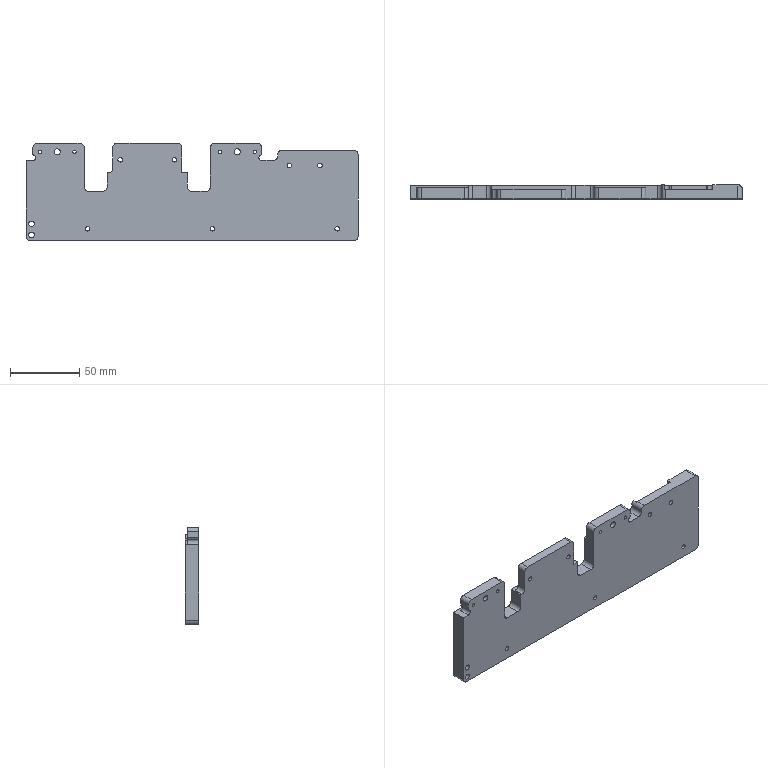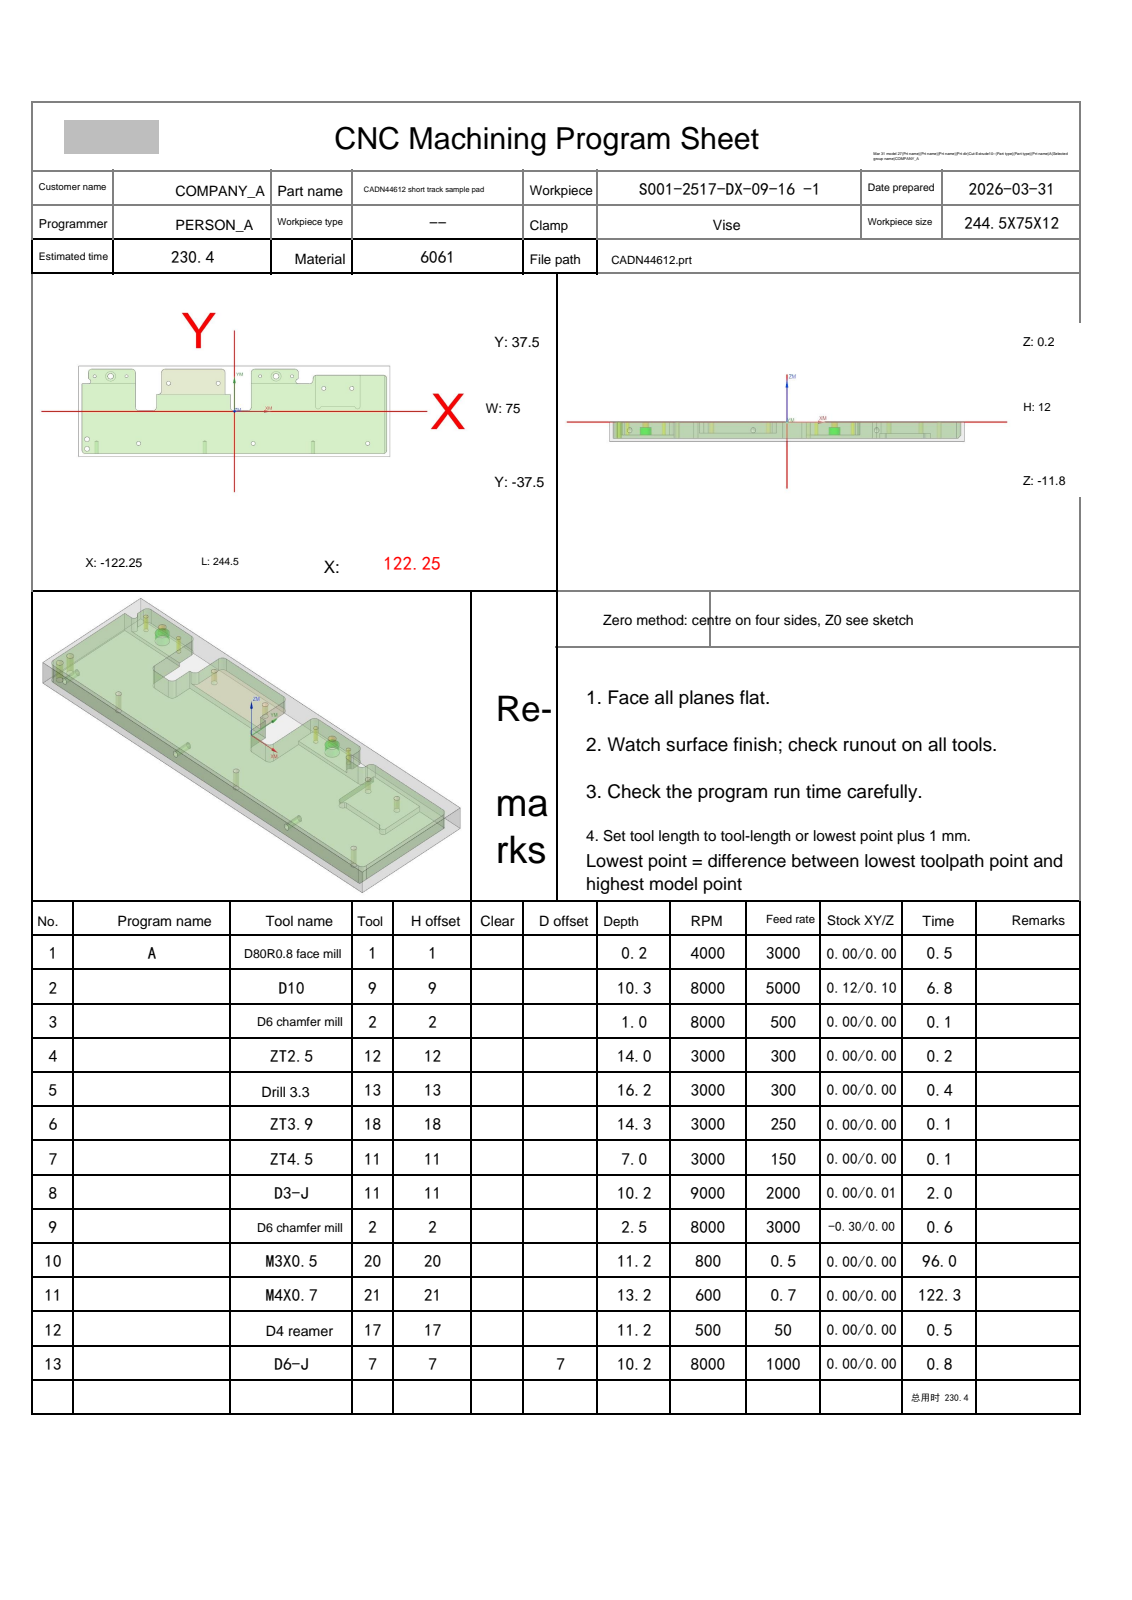NC program | NX | posted by the shop | part box 239.5 x 10 x 70 mm
Lines 1 to 2366 of 10745, first 1729 of 2364 lines:
%
O0001
(Machine time: 433.22 MIN)
(===Total Tool:11===)
(T1=D80R0.8 face mill D=80.  R=0.8  D-  H01 Z=0.    )
(T9=D10     D=10.  R=0.   D-  H09 Z=-10.1 )
(T2=D6 chamfer mill   D=6.   R=0.   D-  H02 Z=-2.3  )
(T12=ZT2.5  D=2.5  DR_a=118 D-  H12 Z=-13.75)
(T13=drill 3.3  D=3.3  DR_a=118 D-  H13 Z=-15.99)
(T18=ZT3.9  D=3.9  DR_a=120 D-  H18 Z=-14.13)
(T11=ZT4.5  D=4.5  DR_a=118 D-  H11 Z=-9.95 )
(T20=M3X0.5 D=2.5  DR_a=180 D-  H20 Z=-11.  )
(T21=M4X0.7 D=3.3  DR_a=180 D-  H21 Z=-13.  )
(T17=D4 reamer   D=4.   DR_a=180 D-  H17 Z=-11.  )
(T7=D6-J    D=6.   R=0.   D7  H07 Z=-10.  )
G80 G90 G17 G49 G40
G91 G28 Z0
M01
N1 T01 M06
(D80R0.8 face mill  D=80. R=0.8 H=01 ce=0.20 di=0.10)
G00 G90 G54 X164.75 Y0.0 M03 S4000
G43 H01 Z20.
M08
Z2.1
G01 Z.1 F3000.
X159.75
X-159.75
X-164.75
Z2.1
G00 Z20.
G00 G90 X164.75 Y0.0 M03 S4000
Z20.
Z2.
G01 Z0.0 F1000.
X159.75
X-159.75
X-164.75
Z2.
G00 Z20.
G91 G28 Z0.0
M05
M09
G91 G28 Z0.0
M01
N2 T09 M06
(D10  D=10. R=0. H=09 ce=0.12 di=0.10)
G00 G90 G54 X-74.5 Y49.5 M03 S8000
G43 H09 Z10.2
M08
Z.719
G01 Z-.481 F5000.
Y45.
G03 X-67.5 Y38. I7. J0.0
G01 X-61.641
G02 X-54.25 Y41.52 I7.391 J-6.
G01 X-10.25
G02 X-2.859 Y38. I0.0 J-9.52
G01 X5.734
G02 X6.734 Y37. I0.0 J-1.
G01 X6.72 Y36.833
X5.872 Y31.818
X5.858 Y31.651
G03 X6.294 Y30.826 I1. J0.0
G02 X6.73 Y30.004 I-.564 J-.826
G01 Y8.016
G02 X5.734 Y7.02 I-1. J.004
G01 X4.266
G02 X3.27 Y8.016 I.004 J1.
G01 Y14.
G03 X-.201 Y19.763 I-6.52 J0.0
G02 X-.73 Y20.641 I.471 J.882
G01 Y30.004
G02 X.266 Y31. I1. J-.004
G01 X2.45
G03 X3.421 Y31.762 I0.0 J1.
G01 X4.763 Y37.238
G02 X5.734 Y38. I.971 J-.238
G01 X8.859
G02 X16.25 Y41.52 I7.391 J-6.
G01 X47.25
G02 X54.641 Y38. I0.0 J-9.52
G01 X122.25
G02 X122.75 Y37.5 I0.0 J-.5
G01 Y34.391
G02 X126.27 Y27. I-6. J-7.391
G01 Y-32.065
G02 X116.75 Y-41.52 I-9.52 J.065
G01 X-116.75
G02 X-126.27 Y-32. I0.0 J9.52
G01 Y22.8
G02 X-122.75 Y28.589 I6.52 J0.0
G01 Y37.5
G02 X-122.25 Y38. I.5 J0.0
G01 X-119.141
G02 X-111.75 Y41.52 I7.391 J-6.
G01 X-80.75
G02 X-73.359 Y38. I0.0 J-9.52
G01 X-62.5
G02 X-61.5 Y37. I0.0 J-1.
X-61.537 Y36.729 I-1. J0.0
G01 X-63.733 Y28.927
G03 X-63.77 Y28.657 I.963 J-.271
G01 Y20.641
G02 X-64.299 Y19.763 I-1. J.004
G03 X-67.77 Y14. I3.049 J-5.763
G01 Y8.016
G02 X-68.766 Y7.02 I-1. J.004
G01 X-70.234
G02 X-71.23 Y8.016 I.004 J1.
G01 Y29.511
G03 X-71.675 Y30.215 I-.779 J0.0
G01 X-72.03 Y30.383
X-72.21 Y30.424
G03 X-72.63 Y30.004 I0.0 J-.42
G01 Y5.62
X-66.37
Y14.
G02 X-62.37 Y18.996 I5.12 J0.0
G01 Y32.
G02 X-54.25 Y40.12 I8.12 J0.0
G01 X-10.25
G02 X-2.13 Y32. I0.0 J-8.12
G01 Y18.996
G02 X1.87 Y14. I-1.12 J-4.996
G01 Y5.62
X8.13
Y32.
G02 X16.25 Y40.12 I8.12 J0.0
G01 X47.25
G02 X55.37 Y32. I0.0 J-8.12
G01 Y27.92
X56.682
G02 X64.75 Y35.12 I8.068 J-.92
G01 X116.75
G02 X124.87 Y27. I0.0 J-8.12
G01 Y-32.046
G02 X116.75 Y-40.12 I-8.12 J.046
G01 X-116.75
G02 X-124.87 Y-32. I0.0 J8.12
G01 Y22.8
G02 X-119.87 Y27.919 I5.12 J0.0
G01 Y32.
G02 X-111.75 Y40.12 I8.12 J0.0
G01 X-80.75
G02 X-72.63 Y32. I0.0 J-8.12
G01 Y30.004
G03 X-72.21 Y29.584 I.42 J0.0
G01 X-72.03 Y29.624
X-71.432 Y29.908
G03 X-71.211 Y30.192 I-.172 J.361
G02 X-70.234 Y31. I.981 J-.192
G01 X-64.766
G02 X-64.497 Y30.962 I-.004 J-1.
X-64.069 Y30.713 I-.273 J-.962
G01 Z.719
G00 Z3.
G01 X-74.5 Y49.5 F6000.
G00 Z.238
G01 Z-.962 F5000.
Y45.
G03 X-67.5 Y38. I7. J0.0
G01 X-61.641
G02 X-54.25 Y41.52 I7.391 J-6.
G01 X-10.25
G02 X-2.859 Y38. I0.0 J-9.52
G01 X5.734
G02 X6.734 Y37. I0.0 J-1.
G01 X6.72 Y36.833
X5.872 Y31.818
X5.858 Y31.651
G03 X6.294 Y30.826 I1. J0.0
G02 X6.73 Y30.004 I-.564 J-.826
G01 Y8.016
G02 X5.734 Y7.02 I-1. J.004
G01 X4.266
G02 X3.27 Y8.016 I.004 J1.
G01 Y14.
G03 X-.201 Y19.763 I-6.52 J0.0
G02 X-.73 Y20.641 I.471 J.882
G01 Y30.004
G02 X.266 Y31. I1. J-.004
G01 X2.45
G03 X3.421 Y31.762 I0.0 J1.
G01 X4.763 Y37.238
G02 X5.734 Y38. I.971 J-.238
G01 X8.859
G02 X16.25 Y41.52 I7.391 J-6.
G01 X47.25
G02 X54.641 Y38. I0.0 J-9.52
G01 X122.25
G02 X122.75 Y37.5 I0.0 J-.5
G01 Y34.391
G02 X126.27 Y27. I-6. J-7.391
G01 Y-32.065
G02 X116.75 Y-41.52 I-9.52 J.065
G01 X-116.75
G02 X-126.27 Y-32. I0.0 J9.52
G01 Y22.8
G02 X-122.75 Y28.589 I6.52 J0.0
G01 Y37.5
G02 X-122.25 Y38. I.5 J0.0
G01 X-119.141
G02 X-111.75 Y41.52 I7.391 J-6.
G01 X-80.75
G02 X-73.359 Y38. I0.0 J-9.52
G01 X-62.5
G02 X-61.5 Y37. I0.0 J-1.
X-61.537 Y36.729 I-1. J0.0
G01 X-63.733 Y28.927
G03 X-63.77 Y28.657 I.963 J-.27
G01 Y20.641
G02 X-64.299 Y19.763 I-1. J.004
G03 X-67.77 Y14. I3.049 J-5.763
G01 Y8.016
G02 X-68.766 Y7.02 I-1. J.004
G01 X-70.234
G02 X-71.23 Y8.016 I.004 J1.
G01 Y29.512
G03 X-71.675 Y30.215 I-.779 J0.0
G01 X-72.03 Y30.384
X-72.21 Y30.424
G03 X-72.63 Y30.004 I0.0 J-.42
G01 Y5.62
X-66.37
Y14.
G02 X-62.37 Y18.996 I5.12 J0.0
G01 Y32.
G02 X-54.25 Y40.12 I8.12 J0.0
G01 X-10.25
G02 X-2.13 Y32. I0.0 J-8.12
G01 Y18.996
G02 X1.87 Y14. I-1.12 J-4.996
G01 Y5.62
X8.13
Y32.
G02 X16.25 Y40.12 I8.12 J0.0
G01 X47.25
G02 X55.37 Y32. I0.0 J-8.12
G01 Y27.92
X56.682
G02 X64.75 Y35.12 I8.068 J-.92
G01 X116.75
G02 X124.87 Y27. I0.0 J-8.12
G01 Y-32.046
G02 X116.75 Y-40.12 I-8.12 J.046
G01 X-116.75
G02 X-124.87 Y-32. I0.0 J8.12
G01 Y22.8
G02 X-119.87 Y27.919 I5.12 J0.0
G01 Y32.
G02 X-111.75 Y40.12 I8.12 J0.0
G01 X-80.75
G02 X-72.63 Y32. I0.0 J-8.12
G01 Y30.004
G03 X-72.21 Y29.584 I.42 J0.0
G01 X-72.03 Y29.625
X-71.432 Y29.908
G03 X-71.211 Y30.192 I-.172 J.361
G02 X-70.234 Y31. I.981 J-.192
G01 X-64.766
G02 X-64.497 Y30.962 I-.004 J-1.
X-64.069 Y30.713 I-.273 J-.962
G01 Z.238
G00 Z2.519
G01 X-74.5 Y49.5 F6000.
G00 Z-.243
G01 Z-1.443 F5000.
Y45.
G03 X-67.5 Y38. I7. J0.0
G01 X-61.641
G02 X-54.25 Y41.52 I7.391 J-6.
G01 X-10.25
G02 X-2.859 Y38. I0.0 J-9.52
G01 X5.734
G02 X6.734 Y37. I0.0 J-1.
G01 X6.72 Y36.833
X5.873 Y31.817
X5.859 Y31.651
G03 X6.294 Y30.826 I1. J0.0
G02 X6.73 Y30.004 I-.564 J-.826
G01 Y8.016
G02 X5.734 Y7.02 I-1. J.004
G01 X4.266
G02 X3.27 Y8.016 I.004 J1.
G01 Y14.
G03 X-.202 Y19.764 I-6.52 J0.0
G02 X-.73 Y20.641 I.472 J.882
G01 Y30.004
G02 X.266 Y31. I1. J-.004
G01 X2.45
G03 X3.421 Y31.762 I0.0 J1.
G01 X4.763 Y37.238
G02 X5.734 Y38. I.971 J-.238
G01 X8.859
G02 X16.25 Y41.52 I7.391 J-6.
G01 X47.25
G02 X54.641 Y38. I0.0 J-9.52
G01 X122.25
G02 X122.75 Y37.5 I0.0 J-.5
G01 Y34.391
G02 X126.27 Y27. I-6. J-7.391
G01 Y-32.065
G02 X116.75 Y-41.52 I-9.52 J.065
G01 X-116.75
G02 X-126.27 Y-32. I0.0 J9.52
G01 Y22.8
G02 X-122.75 Y28.589 I6.52 J0.0
G01 Y37.5
G02 X-122.25 Y38. I.5 J0.0
G01 X-119.141
G02 X-111.75 Y41.52 I7.391 J-6.
G01 X-80.75
G02 X-73.359 Y38. I0.0 J-9.52
G01 X-62.5
G02 X-61.5 Y37. I0.0 J-1.
X-61.537 Y36.729 I-1. J0.0
G01 X-63.733 Y28.927
G03 X-63.77 Y28.657 I.963 J-.271
G01 Y20.641
G02 X-64.298 Y19.764 I-1. J.004
G03 X-67.77 Y14. I3.048 J-5.764
G01 Y8.016
G02 X-68.766 Y7.02 I-1. J.004
G01 X-70.234
G02 X-71.23 Y8.016 I.004 J1.
G01 Y29.512
G03 X-71.675 Y30.215 I-.779 J0.0
G01 X-72.03 Y30.384
X-72.21 Y30.424
G03 X-72.63 Y30.004 I0.0 J-.42
G01 Y5.62
X-66.37
Y14.
G02 X-62.37 Y18.996 I5.12 J0.0
G01 Y32.
G02 X-54.25 Y40.12 I8.12 J0.0
G01 X-10.25
G02 X-2.13 Y32. I0.0 J-8.12
G01 Y18.996
G02 X1.87 Y14. I-1.12 J-4.996
G01 Y5.62
X8.13
Y32.
G02 X16.25 Y40.12 I8.12 J0.0
G01 X47.25
G02 X55.37 Y32. I0.0 J-8.12
G01 Y27.92
X56.682
G02 X64.75 Y35.12 I8.068 J-.92
G01 X116.75
G02 X124.87 Y27. I0.0 J-8.12
G01 Y-32.046
G02 X116.75 Y-40.12 I-8.12 J.046
G01 X-116.75
G02 X-124.87 Y-32. I0.0 J8.12
G01 Y22.8
G02 X-119.87 Y27.919 I5.12 J0.0
G01 Y32.
G02 X-111.75 Y40.12 I8.12 J0.0
G01 X-80.75
G02 X-72.63 Y32. I0.0 J-8.12
G01 Y30.004
G03 X-72.21 Y29.584 I.42 J0.0
G01 X-72.03 Y29.625
X-71.432 Y29.909
G03 X-71.211 Y30.193 I-.172 J.361
G02 X-70.234 Y31. I.981 J-.193
G01 X-64.766
G02 X-64.497 Y30.962 I-.004 J-1.
X-64.069 Y30.713 I-.273 J-.962
G01 Z-.243
G00 Z2.038
G01 X-74.5 Y49.5 F6000.
G00 Z-.724
G01 Z-1.924 F5000.
Y45.
G03 X-67.5 Y38. I7. J0.0
G01 X-61.641
G02 X-54.25 Y41.52 I7.391 J-6.
G01 X-10.25
G02 X-2.859 Y38. I0.0 J-9.52
G01 X5.735
G02 X6.735 Y37. I0.0 J-1.
G01 X6.721 Y36.833
X5.873 Y31.817
X5.859 Y31.651
G03 X6.294 Y30.826 I1. J0.0
G02 X6.73 Y30.005 I-.564 J-.826
G01 Y8.015
G02 X5.735 Y7.02 I-1. J.005
G01 X4.265
G02 X3.27 Y8.015 I.005 J1.
G01 Y14.
G03 X-.202 Y19.764 I-6.52 J0.0
G02 X-.73 Y20.641 I.472 J.882
G01 Y30.005
G02 X.265 Y31. I1. J-.005
G01 X2.45
G03 X3.421 Y31.762 I0.0 J1.
G01 X4.763 Y37.238
G02 X5.735 Y38. I.971 J-.238
G01 X8.859
G02 X16.25 Y41.52 I7.391 J-6.
G01 X47.25
G02 X54.641 Y38. I0.0 J-9.52
G01 X122.25
G02 X122.75 Y37.5 I0.0 J-.5
G01 Y34.391
G02 X126.27 Y27. I-6. J-7.391
G01 Y-32.065
G02 X116.75 Y-41.52 I-9.52 J.065
G01 X-116.75
G02 X-126.27 Y-32. I0.0 J9.52
G01 Y22.8
G02 X-122.75 Y28.589 I6.52 J0.0
G01 Y37.5
G02 X-122.25 Y38. I.5 J0.0
G01 X-119.141
G02 X-111.75 Y41.52 I7.391 J-6.
G01 X-80.75
G02 X-73.359 Y38. I0.0 J-9.52
G01 X-62.5
G02 X-61.5 Y37. I0.0 J-1.
X-61.537 Y36.729 I-1. J0.0
G01 X-63.733 Y28.927
G03 X-63.77 Y28.657 I.963 J-.27
G01 Y20.641
G02 X-64.298 Y19.764 I-1. J.005
G03 X-67.77 Y14. I3.048 J-5.764
G01 Y8.015
G02 X-68.765 Y7.02 I-1. J.005
G01 X-70.235
G02 X-71.23 Y8.015 I.005 J1.
G01 Y29.512
G03 X-71.675 Y30.216 I-.779 J0.0
G01 X-72.03 Y30.384
X-72.21 Y30.425
G03 X-72.63 Y30.005 I0.0 J-.42
G01 Y5.62
X-66.37
Y14.
G02 X-62.37 Y18.996 I5.12 J0.0
G01 Y32.
G02 X-54.25 Y40.12 I8.12 J0.0
G01 X-10.25
G02 X-2.13 Y32. I0.0 J-8.12
G01 Y18.996
G02 X1.87 Y14. I-1.12 J-4.996
G01 Y5.62
X8.13
Y32.
G02 X16.25 Y40.12 I8.12 J0.0
G01 X47.25
G02 X55.37 Y32. I0.0 J-8.12
G01 Y27.92
X56.682
G02 X64.75 Y35.12 I8.068 J-.92
G01 X116.75
G02 X124.87 Y27. I0.0 J-8.12
G01 Y-32.046
G02 X116.75 Y-40.12 I-8.12 J.046
G01 X-116.75
G02 X-124.87 Y-32. I0.0 J8.12
G01 Y22.8
G02 X-119.87 Y27.919 I5.12 J0.0
G01 Y32.
G02 X-111.75 Y40.12 I8.12 J0.0
G01 X-80.75
G02 X-72.63 Y32. I0.0 J-8.12
G01 Y30.005
G03 X-72.21 Y29.585 I.42 J0.0
G01 X-72.03 Y29.625
X-71.432 Y29.909
G03 X-71.211 Y30.193 I-.172 J.361
G02 X-70.235 Y31. I.981 J-.193
G01 X-64.765
G02 X-64.497 Y30.962 I-.005 J-1.
X-64.069 Y30.713 I-.273 J-.962
G01 Z-.724
G00 Z1.557
G01 X-74.5 Y49.5 F6000.
G00 Z-1.205
G01 Z-2.405 F5000.
Y45.
G03 X-67.5 Y38. I7. J0.0
G01 X-61.641
G02 X-54.25 Y41.52 I7.391 J-6.
G01 X-10.25
G02 X-2.859 Y38. I0.0 J-9.52
G01 X5.735
G02 X6.735 Y37. I0.0 J-1.
G01 X6.721 Y36.833
X5.873 Y31.817
X5.859 Y31.651
G03 X6.294 Y30.826 I1. J0.0
G02 X6.73 Y30.005 I-.564 J-.826
G01 Y8.015
G02 X5.735 Y7.02 I-1. J.005
G01 X4.265
G02 X3.27 Y8.015 I.005 J1.
G01 Y14.
G03 X-.202 Y19.764 I-6.52 J0.0
G02 X-.73 Y20.64 I.472 J.882
G01 Y30.005
G02 X.265 Y31. I1. J-.005
G01 X2.451
G03 X3.422 Y31.762 I0.0 J1.
G01 X4.764 Y37.238
G02 X5.735 Y38. I.971 J-.238
G01 X8.859
G02 X16.25 Y41.52 I7.391 J-6.
G01 X47.25
G02 X54.641 Y38. I0.0 J-9.52
G01 X122.25
G02 X122.75 Y37.5 I0.0 J-.5
G01 Y34.391
G02 X126.27 Y27. I-6. J-7.391
G01 Y-32.065
G02 X116.75 Y-41.52 I-9.52 J.065
G01 X-116.75
G02 X-126.27 Y-32. I0.0 J9.52
G01 Y22.8
G02 X-122.75 Y28.589 I6.52 J0.0
G01 Y37.5
G02 X-122.25 Y38. I.5 J0.0
G01 X-119.141
G02 X-111.75 Y41.52 I7.391 J-6.
G01 X-80.75
G02 X-73.359 Y38. I0.0 J-9.52
G01 X-62.5
G02 X-61.5 Y37. I0.0 J-1.
X-61.537 Y36.729 I-1. J0.0
G01 X-63.733 Y28.927
G03 X-63.77 Y28.657 I.963 J-.27
G01 Y20.64
G02 X-64.298 Y19.764 I-1. J.005
G03 X-67.77 Y14. I3.048 J-5.764
G01 Y8.015
G02 X-68.765 Y7.02 I-1. J.005
G01 X-70.235
G02 X-71.23 Y8.015 I.005 J1.
G01 Y29.513
G03 X-71.675 Y30.216 I-.779 J0.0
G01 X-72.03 Y30.384
X-72.21 Y30.425
G03 X-72.63 Y30.005 I0.0 J-.42
G01 Y5.62
X-66.37
Y14.
G02 X-62.37 Y18.996 I5.12 J0.0
G01 Y32.
G02 X-54.25 Y40.12 I8.12 J0.0
G01 X-10.25
G02 X-2.13 Y32. I0.0 J-8.12
G01 Y18.996
G02 X1.87 Y14. I-1.12 J-4.996
G01 Y5.62
X8.13
Y32.
G02 X16.25 Y40.12 I8.12 J0.0
G01 X47.25
G02 X55.37 Y32. I0.0 J-8.12
G01 Y27.92
X56.682
G02 X64.75 Y35.12 I8.068 J-.92
G01 X116.75
G02 X124.87 Y27. I0.0 J-8.12
G01 Y-32.046
G02 X116.75 Y-40.12 I-8.12 J.046
G01 X-116.75
G02 X-124.87 Y-32. I0.0 J8.12
G01 Y22.8
G02 X-119.87 Y27.919 I5.12 J0.0
G01 Y32.
G02 X-111.75 Y40.12 I8.12 J0.0
G01 X-80.75
G02 X-72.63 Y32. I0.0 J-8.12
G01 Y30.005
G03 X-72.21 Y29.585 I.42 J0.0
G01 X-72.03 Y29.625
X-71.432 Y29.909
G03 X-71.211 Y30.193 I-.172 J.361
G02 X-70.235 Y31. I.981 J-.193
G01 X-64.765
G02 X-64.497 Y30.962 I-.005 J-1.
X-64.069 Y30.713 I-.273 J-.962
G01 Z-1.205
G00 Z1.076
G01 X-74.5 Y49.5 F6000.
G00 Z-1.686
G01 Z-2.886 F5000.
Y45.
G03 X-67.5 Y38. I7. J0.0
G01 X-61.641
G02 X-54.25 Y41.52 I7.391 J-6.
G01 X-10.25
G02 X-2.859 Y38. I0.0 J-9.52
G01 X5.735
G02 X6.735 Y37. I0.0 J-1.
G01 X6.721 Y36.833
X5.873 Y31.817
X5.859 Y31.651
G03 X6.294 Y30.826 I1. J0.0
G02 X6.73 Y30.005 I-.564 J-.825
G01 Y8.015
G02 X5.735 Y7.02 I-1. J.005
G01 X4.265
G02 X3.27 Y8.015 I.005 J1.
G01 Y14.
G03 X-.202 Y19.764 I-6.52 J0.0
G02 X-.73 Y20.64 I.472 J.881
G01 Y30.005
G02 X.265 Y31. I1. J-.005
G01 X2.451
G03 X3.422 Y31.762 I0.0 J1.
G01 X4.764 Y37.238
G02 X5.735 Y38. I.971 J-.238
G01 X8.859
G02 X16.25 Y41.52 I7.391 J-6.
G01 X47.25
G02 X54.641 Y38. I0.0 J-9.52
G01 X122.25
G02 X122.75 Y37.5 I0.0 J-.5
G01 Y34.391
G02 X126.27 Y27. I-6. J-7.391
G01 Y-32.065
G02 X116.75 Y-41.52 I-9.52 J.065
G01 X-116.75
G02 X-126.27 Y-32. I0.0 J9.52
G01 Y22.8
G02 X-122.75 Y28.589 I6.52 J0.0
G01 Y37.5
G02 X-122.25 Y38. I.5 J0.0
G01 X-119.141
G02 X-111.75 Y41.52 I7.391 J-6.
G01 X-80.75
G02 X-73.359 Y38. I0.0 J-9.52
G01 X-62.5
G02 X-61.5 Y37. I0.0 J-1.
X-61.537 Y36.729 I-1. J0.0
G01 X-63.733 Y28.927
G03 X-63.77 Y28.657 I.963 J-.271
G01 Y20.64
G02 X-64.298 Y19.764 I-1. J.005
G03 X-67.77 Y14. I3.048 J-5.764
G01 Y8.015
G02 X-68.765 Y7.02 I-1. J.005
G01 X-70.235
G02 X-71.23 Y8.015 I.005 J1.
G01 Y29.513
G03 X-71.675 Y30.216 I-.779 J0.0
G01 X-72.03 Y30.385
X-72.21 Y30.425
G03 X-72.63 Y30.005 I0.0 J-.42
G01 Y5.62
X-66.37
Y14.
G02 X-62.37 Y18.996 I5.12 J0.0
G01 Y32.
G02 X-54.25 Y40.12 I8.12 J0.0
G01 X-10.25
G02 X-2.13 Y32. I0.0 J-8.12
G01 Y18.996
G02 X1.87 Y14. I-1.12 J-4.996
G01 Y5.62
X8.13
Y32.
G02 X16.25 Y40.12 I8.12 J0.0
G01 X47.25
G02 X55.37 Y32. I0.0 J-8.12
G01 Y27.92
X56.682
G02 X64.75 Y35.12 I8.068 J-.92
G01 X116.75
G02 X124.87 Y27. I0.0 J-8.12
G01 Y-32.046
G02 X116.75 Y-40.12 I-8.12 J.046
G01 X-116.75
G02 X-124.87 Y-32. I0.0 J8.12
G01 Y22.8
G02 X-119.87 Y27.919 I5.12 J0.0
G01 Y32.
G02 X-111.75 Y40.12 I8.12 J0.0
G01 X-80.75
G02 X-72.63 Y32. I0.0 J-8.12
G01 Y30.005
G03 X-72.21 Y29.585 I.42 J0.0
G01 X-72.03 Y29.626
X-71.432 Y29.909
G03 X-71.211 Y30.193 I-.172 J.361
G02 X-70.235 Y31. I.981 J-.193
G01 X-64.765
G02 X-64.497 Y30.962 I-.005 J-1.
X-64.069 Y30.713 I-.273 J-.962
G01 Z-1.686
G00 Z.595
G01 X-74.5 Y49.5 F6000.
G00 Z-2.167
G01 Z-3.367 F5000.
Y45.
G03 X-67.5 Y38. I7. J0.0
G01 X-61.641
G02 X-54.25 Y41.52 I7.391 J-6.
G01 X-10.25
G02 X-2.859 Y38. I0.0 J-9.52
G01 X5.735
G02 X6.735 Y37. I0.0 J-1.
G01 X6.721 Y36.833
X5.873 Y31.817
X5.86 Y31.651
G03 X6.295 Y30.825 I1. J0.0
G02 X6.73 Y30.005 I-.565 J-.825
G01 Y8.015
G02 X5.735 Y7.02 I-1. J.005
G01 X4.265
G02 X3.27 Y8.015 I.005 J1.
G01 Y14.
G03 X-.203 Y19.764 I-6.52 J0.0
G02 X-.73 Y20.64 I.473 J.881
G01 Y30.005
G02 X.265 Y31. I1. J-.005
G01 X2.451
G03 X3.422 Y31.762 I0.0 J1.
G01 X4.764 Y37.238
G02 X5.735 Y38. I.971 J-.238
G01 X8.859
G02 X16.25 Y41.52 I7.391 J-6.
G01 X47.25
G02 X54.641 Y38. I0.0 J-9.52
G01 X122.25
G02 X122.75 Y37.5 I0.0 J-.5
G01 Y34.391
G02 X126.27 Y27. I-6. J-7.391
G01 Y-32.065
G02 X116.75 Y-41.52 I-9.52 J.065
G01 X-116.75
G02 X-126.27 Y-32. I0.0 J9.52
G01 Y22.8
G02 X-122.75 Y28.589 I6.52 J0.0
G01 Y37.5
G02 X-122.25 Y38. I.5 J0.0
G01 X-119.141
G02 X-111.75 Y41.52 I7.391 J-6.
G01 X-80.75
G02 X-73.359 Y38. I0.0 J-9.52
G01 X-62.5
G02 X-61.5 Y37. I0.0 J-1.
X-61.537 Y36.729 I-1. J0.0
G01 X-63.733 Y28.927
G03 X-63.77 Y28.657 I.963 J-.271
G01 Y20.64
G02 X-64.297 Y19.764 I-1. J.005
G03 X-67.77 Y14. I3.047 J-5.764
G01 Y8.015
G02 X-68.765 Y7.02 I-1. J.005
G01 X-70.235
G02 X-71.23 Y8.015 I.005 J1.
G01 Y29.513
G03 X-71.675 Y30.216 I-.779 J0.0
G01 X-72.03 Y30.385
X-72.21 Y30.425
G03 X-72.63 Y30.005 I0.0 J-.42
G01 Y5.62
X-66.37
Y14.
G02 X-62.37 Y18.996 I5.12 J0.0
G01 Y32.
G02 X-54.25 Y40.12 I8.12 J0.0
G01 X-10.25
G02 X-2.13 Y32. I0.0 J-8.12
G01 Y18.996
G02 X1.87 Y14. I-1.12 J-4.996
G01 Y5.62
X8.13
Y32.
G02 X16.25 Y40.12 I8.12 J0.0
G01 X47.25
G02 X55.37 Y32. I0.0 J-8.12
G01 Y27.92
X56.682
G02 X64.75 Y35.12 I8.068 J-.92
G01 X116.75
G02 X124.87 Y27. I0.0 J-8.12
G01 Y-32.046
G02 X116.75 Y-40.12 I-8.12 J.046
G01 X-116.75
G02 X-124.87 Y-32. I0.0 J8.12
G01 Y22.8
G02 X-119.87 Y27.919 I5.12 J0.0
G01 Y32.
G02 X-111.75 Y40.12 I8.12 J0.0
G01 X-80.75
G02 X-72.63 Y32. I0.0 J-8.12
G01 Y30.005
G03 X-72.21 Y29.585 I.42 J0.0
G01 X-72.03 Y29.626
X-71.432 Y29.91
G03 X-71.211 Y30.193 I-.172 J.361
G02 X-70.235 Y31. I.981 J-.193
G01 X-64.765
G02 X-64.497 Y30.962 I-.005 J-1.
X-64.069 Y30.713 I-.273 J-.962
G01 Z-2.167
G00 Z.114
G01 X-74.5 Y49.5 F6000.
G00 Z-2.648
G01 Z-3.848 F5000.
Y45.
G03 X-67.5 Y38. I7. J0.0
G01 X-61.641
G02 X-54.25 Y41.52 I7.391 J-6.
G01 X-10.25
G02 X-2.859 Y38. I0.0 J-9.52
G01 X5.736
G02 X6.736 Y37. I0.0 J-1.
G01 X6.722 Y36.833
X5.874 Y31.817
X5.86 Y31.65
G03 X6.295 Y30.825 I1. J0.0
G02 X6.73 Y30.006 I-.565 J-.825
G01 Y8.014
G02 X5.736 Y7.02 I-1. J.006
G01 X4.264
G02 X3.27 Y8.014 I.006 J1.
G01 Y14.
G03 X-.203 Y19.764 I-6.52 J0.0
G02 X-.73 Y20.64 I.473 J.881
G01 Y30.006
G02 X.264 Y31. I1. J-.006
G01 X2.451
G03 X3.422 Y31.762 I0.0 J1.
G01 X4.764 Y37.238
G02 X5.736 Y38. I.971 J-.238
G01 X8.859
G02 X16.25 Y41.52 I7.391 J-6.
G01 X47.25
G02 X54.641 Y38. I0.0 J-9.52
G01 X122.25
G02 X122.75 Y37.5 I0.0 J-.5
G01 Y34.391
G02 X126.27 Y27. I-6. J-7.391
G01 Y-32.065
G02 X116.75 Y-41.52 I-9.52 J.065
G01 X-116.75
G02 X-126.27 Y-32. I0.0 J9.52
G01 Y22.8
G02 X-122.75 Y28.589 I6.52 J0.0
G01 Y37.5
G02 X-122.25 Y38. I.5 J0.0
G01 X-119.141
G02 X-111.75 Y41.52 I7.391 J-6.
G01 X-80.75
G02 X-73.359 Y38. I0.0 J-9.52
G01 X-62.5
G02 X-61.5 Y37. I0.0 J-1.
X-61.537 Y36.729 I-1. J0.0
G01 X-63.733 Y28.927
G03 X-63.77 Y28.657 I.963 J-.271
G01 Y20.64
G02 X-64.297 Y19.764 I-1. J.006
G03 X-67.77 Y14. I3.047 J-5.764
G01 Y8.014
G02 X-68.764 Y7.02 I-1. J.006
G01 X-70.236
G02 X-71.23 Y8.014 I.006 J1.
G01 Y29.513
G03 X-71.675 Y30.217 I-.779 J0.0
G01 X-72.03 Y30.385
X-72.21 Y30.426
G03 X-72.63 Y30.006 I0.0 J-.42
G01 Y5.62
X-66.37
Y14.
G02 X-62.37 Y18.996 I5.12 J0.0
G01 Y32.
G02 X-54.25 Y40.12 I8.12 J0.0
G01 X-10.25
G02 X-2.13 Y32. I0.0 J-8.12
G01 Y18.996
G02 X1.87 Y14. I-1.12 J-4.996
G01 Y5.62
X8.13
Y32.
G02 X16.25 Y40.12 I8.12 J0.0
G01 X47.25
G02 X55.37 Y32. I0.0 J-8.12
G01 Y27.92
X56.682
G02 X64.75 Y35.12 I8.068 J-.92
G01 X116.75
G02 X124.87 Y27. I0.0 J-8.12
G01 Y-32.046
G02 X116.75 Y-40.12 I-8.12 J.046
G01 X-116.75
G02 X-124.87 Y-32. I0.0 J8.12
G01 Y22.8
G02 X-119.87 Y27.919 I5.12 J0.0
G01 Y32.
G02 X-111.75 Y40.12 I8.12 J0.0
G01 X-80.75
G02 X-72.63 Y32. I0.0 J-8.12
G01 Y30.006
G03 X-72.21 Y29.586 I.42 J0.0
G01 X-72.03 Y29.626
X-71.432 Y29.91
G03 X-71.211 Y30.194 I-.172 J.361
G02 X-70.236 Y31. I.981 J-.194
G01 X-64.764
G02 X-64.497 Y30.962 I-.006 J-1.
X-64.069 Y30.713 I-.273 J-.962
G01 Z-2.648
G00 Z-.367
G01 X-74.5 Y49.5 F6000.
G00 Z-3.129
G01 Z-4.329 F5000.
Y45.
G03 X-67.5 Y38. I7. J0.0
G01 X-61.641
G02 X-54.25 Y41.52 I7.391 J-6.
G01 X-10.25
G02 X-2.859 Y38. I0.0 J-9.52
G01 X5.736
G02 X6.736 Y37. I0.0 J-1.
G01 X6.722 Y36.833
X5.874 Y31.817
X5.86 Y31.65
G03 X6.295 Y30.825 I1. J0.0
G02 X6.73 Y30.006 I-.565 J-.825
G01 Y8.014
G02 X5.736 Y7.02 I-1. J.006
G01 X4.264
G02 X3.27 Y8.014 I.006 J1.
G01 Y14.
G03 X-.203 Y19.764 I-6.52 J0.0
G02 X-.73 Y20.639 I.473 J.881
G01 Y30.006
G02 X.264 Y31. I1. J-.006
G01 X2.452
G03 X3.423 Y31.762 I0.0 J1.
G01 X4.765 Y37.238
G02 X5.736 Y38. I.971 J-.238
G01 X8.859
G02 X16.25 Y41.52 I7.391 J-6.
G01 X47.25
G02 X54.641 Y38. I0.0 J-9.52
G01 X122.25
G02 X122.75 Y37.5 I0.0 J-.5
G01 Y34.391
G02 X126.27 Y27. I-6. J-7.391
G01 Y-32.065
G02 X116.75 Y-41.52 I-9.52 J.065
G01 X-116.75
G02 X-126.27 Y-32. I0.0 J9.52
G01 Y22.8
G02 X-122.75 Y28.589 I6.52 J0.0
G01 Y37.5
G02 X-122.25 Y38. I.5 J0.0
G01 X-119.141
G02 X-111.75 Y41.52 I7.391 J-6.
G01 X-80.75
G02 X-73.359 Y38. I0.0 J-9.52
G01 X-62.5
G02 X-61.5 Y37. I0.0 J-1.
X-61.537 Y36.729 I-1. J0.0
G01 X-63.733 Y28.927
G03 X-63.77 Y28.657 I.963 J-.271
G01 Y20.639
G02 X-64.297 Y19.764 I-1. J.006
G03 X-67.77 Y14. I3.047 J-5.764
G01 Y8.014
G02 X-68.764 Y7.02 I-1. J.006
G01 X-70.236
G02 X-71.23 Y8.014 I.006 J1.
G01 Y29.513
G03 X-71.675 Y30.217 I-.779 J0.0
G01 X-72.03 Y30.385
X-72.21 Y30.426
G03 X-72.63 Y30.006 I0.0 J-.42
G01 Y5.62
X-66.37
Y14.
G02 X-62.37 Y18.996 I5.12 J0.0
G01 Y32.
G02 X-54.25 Y40.12 I8.12 J0.0
G01 X-10.25
G02 X-2.13 Y32. I0.0 J-8.12
G01 Y18.996
G02 X1.87 Y14. I-1.12 J-4.996
G01 Y5.62
X8.13
Y32.
G02 X16.25 Y40.12 I8.12 J0.0
G01 X47.25
G02 X55.37 Y32. I0.0 J-8.12
G01 Y27.92
X56.682
G02 X64.75 Y35.12 I8.068 J-.92
G01 X116.75
G02 X124.87 Y27. I0.0 J-8.12
G01 Y-32.046
G02 X116.75 Y-40.12 I-8.12 J.046
G01 X-116.75
G02 X-124.87 Y-32. I0.0 J8.12
G01 Y22.8
G02 X-119.87 Y27.919 I5.12 J0.0
G01 Y32.
G02 X-111.75 Y40.12 I8.12 J0.0
G01 X-80.75
G02 X-72.63 Y32. I0.0 J-8.12
G01 Y30.006
G03 X-72.21 Y29.586 I.42 J0.0
G01 X-72.03 Y29.626
X-71.432 Y29.91
G03 X-71.211 Y30.194 I-.172 J.361
G02 X-70.236 Y31. I.981 J-.194
G01 X-64.764
G02 X-64.497 Y30.962 I-.006 J-1.
X-64.069 Y30.713 I-.273 J-.962
G01 Z-3.129
G00 Z-.848
G01 X-74.5 Y49.5 F6000.
G00 Z-3.61
G01 Z-4.81 F5000.
Y45.
G03 X-67.5 Y38. I7. J0.0
G01 X-61.641
G02 X-54.25 Y41.52 I7.391 J-6.
G01 X-10.25
G02 X-2.859 Y38. I0.0 J-9.52
G01 X5.736
G02 X6.736 Y37. I0.0 J-1.
G01 X6.722 Y36.833
X5.874 Y31.816
X5.86 Y31.65
G03 X6.295 Y30.825 I1. J0.0
G02 X6.73 Y30.006 I-.565 J-.825
G01 Y8.014
G02 X5.736 Y7.02 I-1. J.006
G01 X4.264
G02 X3.27 Y8.014 I.006 J1.
G01 Y14.
G03 X-.203 Y19.764 I-6.52 J0.0
G02 X-.73 Y20.639 I.473 J.881
G01 Y30.006
G02 X.264 Y31. I1. J-.006
G01 X2.452
G03 X3.423 Y31.762 I0.0 J1.
G01 X4.765 Y37.238
G02 X5.736 Y38. I.971 J-.238
G01 X8.859
G02 X16.25 Y41.52 I7.391 J-6.
G01 X47.25
G02 X54.641 Y38. I0.0 J-9.52
G01 X122.25
G02 X122.75 Y37.5 I0.0 J-.5
G01 Y34.391
G02 X126.27 Y27. I-6. J-7.391
G01 Y-32.065
G02 X116.75 Y-41.52 I-9.52 J.065
G01 X-116.75
G02 X-126.27 Y-32. I0.0 J9.52
G01 Y22.8
G02 X-122.75 Y28.589 I6.52 J0.0
G01 Y37.5
G02 X-122.25 Y38. I.5 J0.0
G01 X-119.141
G02 X-111.75 Y41.52 I7.391 J-6.
G01 X-80.75
G02 X-73.359 Y38. I0.0 J-9.52
G01 X-62.5
G02 X-61.5 Y37. I0.0 J-1.
X-61.537 Y36.729 I-1. J0.0
G01 X-63.733 Y28.927
G03 X-63.77 Y28.657 I.963 J-.271
G01 Y20.639
G02 X-64.297 Y19.764 I-1. J.006
G03 X-67.77 Y14. I3.047 J-5.764
G01 Y8.014
G02 X-68.764 Y7.02 I-1. J.006
G01 X-70.236
G02 X-71.23 Y8.014 I.006 J1.
G01 Y29.514
G03 X-71.675 Y30.217 I-.779 J0.0
G01 X-72.03 Y30.386
X-72.21 Y30.426
G03 X-72.63 Y30.006 I0.0 J-.42
G01 Y5.62
X-66.37
Y14.
G02 X-62.37 Y18.996 I5.12 J0.0
G01 Y32.
G02 X-54.25 Y40.12 I8.12 J0.0
G01 X-10.25
G02 X-2.13 Y32. I0.0 J-8.12
G01 Y18.996
G02 X1.87 Y14. I-1.12 J-4.996
G01 Y5.62
X8.13
Y32.
G02 X16.25 Y40.12 I8.12 J0.0
G01 X47.25
G02 X55.37 Y32. I0.0 J-8.12
G01 Y27.92
X56.682
G02 X64.75 Y35.12 I8.068 J-.92
G01 X116.75
G02 X124.87 Y27. I0.0 J-8.12
G01 Y-32.046
G02 X116.75 Y-40.12 I-8.12 J.046
G01 X-116.75
G02 X-124.87 Y-32. I0.0 J8.12
G01 Y22.8
G02 X-119.87 Y27.919 I5.12 J0.0
G01 Y32.
G02 X-111.75 Y40.12 I8.12 J0.0
G01 X-80.75
G02 X-72.63 Y32. I0.0 J-8.12
G01 Y30.006
G03 X-72.21 Y29.586 I.42 J0.0
G01 X-72.03 Y29.627
X-71.432 Y29.91
G03 X-71.211 Y30.194 I-.172 J.361
G02 X-70.236 Y31. I.981 J-.194
G01 X-64.764
G02 X-64.497 Y30.962 I-.006 J-1.
X-64.069 Y30.713 I-.273 J-.962
G01 Z-3.61
G00 Z-1.329
G01 X-74.5 Y49.5 F6000.
G00 Z-4.09
G01 Z-5.29 F5000.
Y45.
G03 X-67.5 Y38. I7. J0.0
G01 X-61.641
G02 X-54.25 Y41.52 I7.391 J-6.
G01 X-10.25
G02 X-2.859 Y38. I0.0 J-9.52
G01 X5.736
G02 X6.736 Y37. I0.0 J-1.
G01 X6.722 Y36.833
X5.874 Y31.816
X5.86 Y31.65
G03 X6.295 Y30.825 I1. J0.0
G02 X6.73 Y30.006 I-.565 J-.825
G01 Y8.014
G02 X5.736 Y7.02 I-1. J.006
G01 X4.264
G02 X3.27 Y8.014 I.006 J1.
G01 Y14.
G03 X-.203 Y19.764 I-6.52 J0.0
G02 X-.73 Y20.639 I.473 J.881
G01 Y30.006
G02 X.264 Y31. I1. J-.006
G01 X2.452
G03 X3.423 Y31.762 I0.0 J1.
G01 X4.765 Y37.238
G02 X5.736 Y38. I.971 J-.238
G01 X8.859
G02 X16.25 Y41.52 I7.391 J-6.
G01 X47.25
G02 X54.641 Y38. I0.0 J-9.52
G01 X122.25
G02 X122.75 Y37.5 I0.0 J-.5
G01 Y34.391
G02 X126.27 Y27. I-6. J-7.391
G01 Y-32.065
G02 X116.75 Y-41.52 I-9.52 J.065
G01 X-116.75
G02 X-126.27 Y-32. I0.0 J9.52
G01 Y22.8
G02 X-122.75 Y28.589 I6.52 J0.0
G01 Y37.5
G02 X-122.25 Y38. I.5 J0.0
G01 X-119.141
G02 X-111.75 Y41.52 I7.391 J-6.
G01 X-80.75
G02 X-73.359 Y38. I0.0 J-9.52
G01 X-62.5
G02 X-61.5 Y37. I0.0 J-1.
X-61.537 Y36.729 I-1. J0.0
G01 X-63.733 Y28.927
G03 X-63.77 Y28.657 I.963 J-.271
G01 Y20.639
G02 X-64.297 Y19.764 I-1. J.006
G03 X-67.77 Y14. I3.047 J-5.764
G01 Y8.014
G02 X-68.764 Y7.02 I-1. J.006
G01 X-70.236
G02 X-71.23 Y8.014 I.006 J1.
G01 Y29.514
G03 X-71.675 Y30.217 I-.779 J0.0
G01 X-72.03 Y30.386
X-72.21 Y30.426
G03 X-72.63 Y30.006 I0.0 J-.42
G01 Y5.62
X-66.37
Y14.
G02 X-62.37 Y18.996 I5.12 J0.0
G01 Y32.
G02 X-54.25 Y40.12 I8.12 J0.0
G01 X-10.25
G02 X-2.13 Y32. I0.0 J-8.12
G01 Y18.996
G02 X1.87 Y14. I-1.12 J-4.996
G01 Y5.62
X8.13
Y32.
G02 X16.25 Y40.12 I8.12 J0.0
G01 X47.25
G02 X55.37 Y32. I0.0 J-8.12
G01 Y27.92
X56.682
G02 X64.75 Y35.12 I8.068 J-.92
G01 X116.75
G02 X124.87 Y27. I0.0 J-8.12
G01 Y-32.046
G02 X116.75 Y-40.12 I-8.12 J.046
G01 X-116.75
G02 X-124.87 Y-32. I0.0 J8.12
G01 Y22.8
G02 X-119.87 Y27.919 I5.12 J0.0
G01 Y32.
G02 X-111.75 Y40.12 I8.12 J0.0
G01 X-80.75
G02 X-72.63 Y32. I0.0 J-8.12
G01 Y30.006
G03 X-72.21 Y29.586 I.42 J0.0
G01 X-72.03 Y29.627
X-71.432 Y29.911
G03 X-71.211 Y30.194 I-.172 J.361
G02 X-70.236 Y31. I.981 J-.194
G01 X-64.764
G02 X-64.497 Y30.962 I-.006 J-1.
X-64.069 Y30.713 I-.273 J-.962
G01 Z-4.09
G00 Z-1.81
G01 X-74.5 Y49.5 F6000.
G00 Z-4.571
G01 Z-5.771 F5000.
Y45.
G03 X-67.5 Y38. I7. J0.0
G01 X-61.641
G02 X-54.25 Y41.52 I7.391 J-6.
G01 X-10.25
G02 X-2.859 Y38. I0.0 J-9.52
G01 X5.736
G02 X6.736 Y37. I0.0 J-1.
G01 X6.722 Y36.833
X5.874 Y31.816
X5.86 Y31.65
G03 X6.295 Y30.825 I1. J0.0
G02 X6.73 Y30.006 I-.565 J-.825
G01 Y8.014
G02 X5.736 Y7.02 I-1. J.006
G01 X4.264
G02 X3.27 Y8.014 I.006 J1.
G01 Y14.
G03 X-.203 Y19.764 I-6.52 J0.0
G02 X-.73 Y20.639 I.473 J.881
G01 Y30.006
G02 X.264 Y31. I1. J-.006
G01 X2.452
G03 X3.423 Y31.762 I0.0 J1.
G01 X4.765 Y37.238
G02 X5.736 Y38. I.971 J-.238
G01 X8.859
G02 X16.25 Y41.52 I7.391 J-6.
G01 X47.25
G02 X54.641 Y38. I0.0 J-9.52
G01 X122.25
G02 X122.75 Y37.5 I0.0 J-.5
G01 Y34.391
G02 X126.27 Y27. I-6. J-7.391
G01 Y-32.065
G02 X116.75 Y-41.52 I-9.52 J.065
G01 X-116.75
G02 X-126.27 Y-32. I0.0 J9.52
G01 Y22.8
G02 X-122.75 Y28.589 I6.52 J0.0
G01 Y37.5
G02 X-122.25 Y38. I.5 J0.0
G01 X-119.141
G02 X-111.75 Y41.52 I7.391 J-6.
G01 X-80.75
G02 X-73.359 Y38. I0.0 J-9.52
G01 X-62.5
G02 X-61.5 Y37. I0.0 J-1.
X-61.537 Y36.729 I-1. J0.0
G01 X-63.733 Y28.927
G03 X-63.77 Y28.657 I.963 J-.271
G01 Y20.639
G02 X-64.297 Y19.764 I-1. J.006
G03 X-67.77 Y14. I3.047 J-5.764
G01 Y8.014
G02 X-68.764 Y7.02 I-1. J.006
G01 X-70.236
G02 X-71.23 Y8.014 I.006 J1.
G01 Y29.514
G03 X-71.675 Y30.217 I-.779 J0.0
G01 X-72.03 Y30.386
X-72.21 Y30.426
G03 X-72.63 Y30.006 I0.0 J-.42
G01 Y5.62
X-66.37
Y14.
G02 X-62.37 Y18.996 I5.12 J0.0
G01 Y32.
G02 X-54.25 Y40.12 I8.12 J0.0
G01 X-10.25
G02 X-2.13 Y32. I0.0 J-8.12
G01 Y18.996
G02 X1.87 Y14. I-1.12 J-4.996
G01 Y5.62
X8.13
Y32.
G02 X16.25 Y40.12 I8.12 J0.0
G01 X47.25
G02 X55.37 Y32. I0.0 J-8.12
G01 Y27.92
X56.682
G02 X64.75 Y35.12 I8.068 J-.92
G01 X116.75
G02 X124.87 Y27. I0.0 J-8.12
G01 Y-32.046
G02 X116.75 Y-40.12 I-8.12 J.046
G01 X-116.75
G02 X-124.87 Y-32. I0.0 J8.12
G01 Y22.8
G02 X-119.87 Y27.919 I5.12 J0.0
G01 Y32.
G02 X-111.75 Y40.12 I8.12 J0.0
G01 X-80.75
G02 X-72.63 Y32. I0.0 J-8.12
G01 Y30.006
G03 X-72.21 Y29.586 I.42 J0.0
G01 X-72.03 Y29.627
X-71.432 Y29.911
G03 X-71.211 Y30.194 I-.172 J.361
G02 X-70.236 Y31. I.981 J-.194
G01 X-64.764
G02 X-64.497 Y30.962 I-.006 J-1.
X-64.069 Y30.713 I-.273 J-.962
G01 Z-4.571
G00 Z-2.29
G01 X-74.5 Y49.5 F6000.
G00 Z-5.052
G01 Z-6.252 F5000.
Y45.
G03 X-67.5 Y38. I7. J0.0
G01 X-61.641
G02 X-54.25 Y41.52 I7.391 J-6.
G01 X-10.25
G02 X-2.859 Y38. I0.0 J-9.52
G01 X5.737
G02 X6.737 Y37. I0.0 J-1.
G01 X6.723 Y36.833
X5.875 Y31.816
X5.861 Y31.65
G03 X6.295 Y30.825 I1. J0.0
G02 X6.73 Y30.007 I-.565 J-.825
G01 Y8.013
G02 X5.737 Y7.02 I-1. J.007
G01 X4.263
G02 X3.27 Y8.013 I.007 J1.
G01 Y14.
G03 X-.204 Y19.764 I-6.52 J0.0
G02 X-.73 Y20.639 I.474 J.881
G01 Y30.007
G02 X.263 Y31. I1. J-.007
G01 X2.452
G03 X3.423 Y31.762 I0.0 J1.
G01 X4.765 Y37.238
G02 X5.737 Y38. I.971 J-.238
G01 X8.859
G02 X16.25 Y41.52 I7.391 J-6.
G01 X47.25
G02 X54.641 Y38. I0.0 J-9.52
G01 X122.25
G02 X122.75 Y37.5 I0.0 J-.5
G01 Y34.391
G02 X126.27 Y27. I-6. J-7.391
G01 Y-32.065
G02 X116.75 Y-41.52 I-9.52 J.065
G01 X-116.75
G02 X-126.27 Y-32. I0.0 J9.52
G01 Y22.8
G02 X-122.75 Y28.589 I6.52 J0.0
G01 Y37.5
G02 X-122.25 Y38. I.5 J0.0
G01 X-119.141
G02 X-111.75 Y41.52 I7.391 J-6.
G01 X-80.75
G02 X-73.359 Y38. I0.0 J-9.52
G01 X-62.5
G02 X-61.5 Y37. I0.0 J-1.
X-61.537 Y36.729 I-1. J0.0
G01 X-63.733 Y28.927
G03 X-63.77 Y28.657 I.963 J-.271
G01 Y20.639
G02 X-64.296 Y19.764 I-1. J.007
G03 X-67.77 Y14. I3.046 J-5.764
G01 Y8.013
G02 X-68.763 Y7.02 I-1. J.007
G01 X-70.237
G02 X-71.23 Y8.013 I.007 J1.
G01 Y29.514
G03 X-71.675 Y30.218 I-.779 J0.0
G01 X-72.03 Y30.386
X-72.21 Y30.427
G03 X-72.63 Y30.007 I0.0 J-.42
G01 Y5.62
X-66.37
Y14.
G02 X-62.37 Y18.996 I5.12 J0.0
G01 Y32.
G02 X-54.25 Y40.12 I8.12 J0.0
G01 X-10.25
G02 X-2.13 Y32. I0.0 J-8.12
G01 Y18.996
G02 X1.87 Y14. I-1.12 J-4.996
G01 Y5.62
X8.13
Y32.
G02 X16.25 Y40.12 I8.12 J0.0
G01 X47.25
G02 X55.37 Y32. I0.0 J-8.12
G01 Y27.92
X56.682
G02 X64.75 Y35.12 I8.068 J-.92
G01 X116.75
G02 X124.87 Y27. I0.0 J-8.12
G01 Y-32.046
G02 X116.75 Y-40.12 I-8.12 J.046
G01 X-116.75
G02 X-124.87 Y-32. I0.0 J8.12
G01 Y22.8
G02 X-119.87 Y27.919 I5.12 J0.0
G01 Y32.
G02 X-111.75 Y40.12 I8.12 J0.0
G01 X-80.75
G02 X-72.63 Y32. I0.0 J-8.12
G01 Y30.007
G03 X-72.21 Y29.587 I.42 J0.0
G01 X-72.03 Y29.627
X-71.432 Y29.911
G03 X-71.211 Y30.194 I-.172 J.361
G02 X-70.237 Y31. I.981 J-.194
G01 X-64.763
G02 X-64.497 Y30.962 I-.007 J-1.
X-64.069 Y30.713 I-.273 J-.962
G01 Z-5.052
G00 Z-2.771
G01 X-74.5 Y49.5 F6000.
G00 Z-5.533
G01 Z-6.733 F5000.
Y45.
G03 X-67.5 Y38. I7. J0.0
G01 X-61.641
G02 X-54.25 Y41.52 I7.391 J-6.
G01 X-10.25
G02 X-2.859 Y38. I0.0 J-9.52
G01 X5.737
G02 X6.737 Y37. I0.0 J-1.
G01 X6.723 Y36.833
X5.875 Y31.816
X5.861 Y31.65
G03 X6.295 Y30.825 I1. J0.0
G02 X6.73 Y30.007 I-.565 J-.825
G01 Y8.013
G02 X5.737 Y7.02 I-1. J.007
G01 X4.263
G02 X3.27 Y8.013 I.007 J1.
G01 Y14.
G03 X-.204 Y19.765 I-6.52 J0.0
G02 X-.73 Y20.639 I.474 J.881
G01 Y30.007
G02 X.263 Y31. I1. J-.007
G01 X2.453
G03 X3.423 Y31.762 I0.0 J1.
G01 X4.766 Y37.238
G02 X5.737 Y38. I.971 J-.238
G01 X8.859
G02 X16.25 Y41.52 I7.391 J-6.
G01 X47.25
G02 X54.641 Y38. I0.0 J-9.52
G01 X122.25
G02 X122.75 Y37.5 I0.0 J-.5
G01 Y34.391
G02 X126.27 Y27. I-6. J-7.391
G01 Y-32.065
G02 X116.75 Y-41.52 I-9.52 J.065
G01 X-116.75
G02 X-126.27 Y-32. I0.0 J9.52
G01 Y22.8
G02 X-122.75 Y28.589 I6.52 J0.0
G01 Y37.5
G02 X-122.25 Y38. I.5 J0.0
G01 X-119.141
G02 X-111.75 Y41.52 I7.391 J-6.
G01 X-80.75
G02 X-73.359 Y38. I0.0 J-9.52
G01 X-62.5
G02 X-61.5 Y37. I0.0 J-1.
X-61.537 Y36.729 I-1. J0.0
G01 X-63.733 Y28.927
G03 X-63.77 Y28.657 I.963 J-.271
G01 Y20.639
G02 X-64.296 Y19.765 I-1. J.007
G03 X-67.77 Y14. I3.046 J-5.765
G01 Y8.013
G02 X-68.763 Y7.02 I-1. J.007
G01 X-70.237
G02 X-71.23 Y8.013 I.007 J1.
G01 Y29.514
G03 X-71.675 Y30.218 I-.779 J0.0
G01 X-72.03 Y30.386
X-72.21 Y30.427
G03 X-72.63 Y30.007 I0.0 J-.42
G01 Y5.62
X-66.37
Y14.
G02 X-62.37 Y18.996 I5.12 J0.0
G01 Y32.
G02 X-54.25 Y40.12 I8.12 J0.0
G01 X-10.25
G02 X-2.13 Y32. I0.0 J-8.12
G01 Y18.996
G02 X1.87 Y14. I-1.12 J-4.996
G01 Y5.62
X8.13
Y32.
G02 X16.25 Y40.12 I8.12 J0.0
G01 X47.25
G02 X55.37 Y32. I0.0 J-8.12
G01 Y27.92
X56.682
G02 X64.75 Y35.12 I8.068 J-.92
G01 X116.75
G02 X124.87 Y27. I0.0 J-8.12
G01 Y-32.046
G02 X116.75 Y-40.12 I-8.12 J.046
G01 X-116.75
G02 X-124.87 Y-32. I0.0 J8.12
G01 Y22.8
G02 X-119.87 Y27.919 I5.12 J0.0
G01 Y32.
G02 X-111.75 Y40.12 I8.12 J0.0
G01 X-80.75
G02 X-72.63 Y32. I0.0 J-8.12
G01 Y30.007
G03 X-72.21 Y29.587 I.42 J0.0
G01 X-72.03 Y29.627
X-71.432 Y29.911
G03 X-71.211 Y30.194 I-.172 J.361
G02 X-70.237 Y31. I.981 J-.194
G01 X-64.763
G02 X-64.497 Y30.962 I-.007 J-1.
X-64.069 Y30.713 I-.273 J-.962
G01 Z-5.533
G00 Z-3.252
G01 X-74.5 Y49.5 F6000.
G00 Z-6.014
G01 Z-7.214 F5000.
Y45.
G03 X-67.5 Y38. I7. J0.0
G01 X-61.641
G02 X-54.25 Y41.52 I7.391 J-6.
G01 X-10.25
G02 X-2.859 Y38. I0.0 J-9.52
G01 X5.737
G02 X6.737 Y37. I0.0 J-1.
G01 X6.723 Y36.833
X5.875 Y31.816
X5.861 Y31.65
G03 X6.295 Y30.825 I1. J0.0
G02 X6.73 Y30.007 I-.565 J-.825
G01 Y8.013
G02 X5.737 Y7.02 I-1. J.007
G01 X4.263
G02 X3.27 Y8.013 I.007 J1.
G01 Y14.
G03 X-.204 Y19.765 I-6.52 J0.0
G02 X-.73 Y20.638 I.474 J.881
G01 Y30.007
G02 X.263 Y31. I1. J-.007
G01 X2.453
G03 X3.424 Y31.762 I0.0 J1.
G01 X4.766 Y37.238
G02 X5.737 Y38. I.971 J-.238
G01 X8.859
G02 X16.25 Y41.52 I7.391 J-6.
G01 X47.25
G02 X54.641 Y38. I0.0 J-9.52
G01 X122.25
G02 X122.75 Y37.5 I0.0 J-.5
G01 Y34.391
G02 X126.27 Y27. I-6. J-7.391
G01 Y-32.065
G02 X116.75 Y-41.52 I-9.52 J.065
G01 X-116.75
G02 X-126.27 Y-32. I0.0 J9.52
G01 Y22.8
G02 X-122.75 Y28.589 I6.52 J0.0
G01 Y37.5
G02 X-122.25 Y38. I.5 J0.0
G01 X-119.141
G02 X-111.75 Y41.52 I7.391 J-6.
G01 X-80.75
G02 X-73.359 Y38. I0.0 J-9.52
G01 X-62.5
G02 X-61.5 Y37. I0.0 J-1.
X-61.537 Y36.729 I-1. J0.0
G01 X-63.733 Y28.927
G03 X-63.77 Y28.657 I.963 J-.27
G01 Y20.638
G02 X-64.296 Y19.765 I-1. J.007
G03 X-67.77 Y14. I3.046 J-5.765
G01 Y8.013
G02 X-68.763 Y7.02 I-1. J.007
G01 X-70.237
G02 X-71.23 Y8.013 I.007 J1.
G01 Y29.515
G03 X-71.675 Y30.218 I-.779 J0.0
G01 X-72.03 Y30.386
X-72.21 Y30.427
G03 X-72.63 Y30.007 I0.0 J-.42
G01 Y5.62
X-66.37
Y14.
G02 X-62.37 Y18.996 I5.12 J0.0
G01 Y32.
G02 X-54.25 Y40.12 I8.12 J0.0
G01 X-10.25
G02 X-2.13 Y32. I0.0 J-8.12
G01 Y18.996
G02 X1.87 Y14. I-1.12 J-4.996
G01 Y5.62
X8.13
Y32.
G02 X16.25 Y40.12 I8.12 J0.0
G01 X47.25
G02 X55.37 Y32. I0.0 J-8.12
G01 Y27.92
X56.682
G02 X64.75 Y35.12 I8.068 J-.92
G01 X116.75
G02 X124.87 Y27. I0.0 J-8.12
G01 Y-32.046
G02 X116.75 Y-40.12 I-8.12 J.046
G01 X-116.75
G02 X-124.87 Y-32. I0.0 J8.12
G01 Y22.8
G02 X-119.87 Y27.919 I5.12 J0.0
G01 Y32.
G02 X-111.75 Y40.12 I8.12 J0.0
G01 X-80.75
G02 X-72.63 Y32. I0.0 J-8.12
G01 Y30.007
G03 X-72.21 Y29.587 I.42 J0.0
G01 X-72.03 Y29.628
X-71.432 Y29.911
G03 X-71.211 Y30.195 I-.172 J.361
G02 X-70.237 Y31. I.981 J-.195
G01 X-64.763
G02 X-64.497 Y30.962 I-.007 J-1.
X-64.069 Y30.713 I-.273 J-.962
G01 Z-6.014
G00 Z-3.733
G01 X-74.5 Y49.5 F6000.
G00 Z-6.495
G01 Z-7.695 F5000.
Y45.
G03 X-67.5 Y38. I7. J0.0
G01 X-61.641
G02 X-54.25 Y41.52 I7.391 J-6.
G01 X-10.25
G02 X-2.859 Y38. I0.0 J-9.52
G01 X5.737
G02 X6.737 Y37. I0.0 J-1.
G01 X6.723 Y36.833
X5.875 Y31.816
X5.861 Y31.649
G03 X6.295 Y30.825 I1. J0.0
G02 X6.73 Y30.007 I-.565 J-.825
G01 Y8.013
G02 X5.737 Y7.02 I-1. J.007
G01 X4.263
G02 X3.27 Y8.013 I.007 J1.
G01 Y14.
G03 X-.204 Y19.765 I-6.52 J0.0
G02 X-.73 Y20.638 I.474 J.881
G01 Y30.007
G02 X.263 Y31. I1. J-.007
G01 X2.453
G03 X3.424 Y31.762 I0.0 J1.
G01 X4.766 Y37.238
G02 X5.737 Y38. I.971 J-.238
G01 X8.859
G02 X16.25 Y41.52 I7.391 J-6.
G01 X47.25
G02 X54.641 Y38. I0.0 J-9.52
G01 X122.25
G02 X122.75 Y37.5 I0.0 J-.5
G01 Y34.391
G02 X126.27 Y27. I-6. J-7.391
G01 Y-32.065
G02 X116.75 Y-41.52 I-9.52 J.065
G01 X-116.75
G02 X-126.27 Y-32. I0.0 J9.52
G01 Y22.8
G02 X-122.75 Y28.589 I6.52 J0.0
G01 Y37.5
G02 X-122.25 Y38. I.5 J0.0
G01 X-119.141
G02 X-111.75 Y41.52 I7.391 J-6.
G01 X-80.75
G02 X-73.359 Y38. I0.0 J-9.52
G01 X-62.5
G02 X-61.5 Y37. I0.0 J-1.
X-61.537 Y36.729 I-1. J0.0
G01 X-63.733 Y28.927
G03 X-63.77 Y28.657 I.963 J-.271
G01 Y20.638
G02 X-64.296 Y19.765 I-1. J.007
G03 X-67.77 Y14. I3.046 J-5.765
G01 Y8.013
G02 X-68.763 Y7.02 I-1. J.007
G01 X-70.237
G02 X-71.23 Y8.013 I.007 J1.